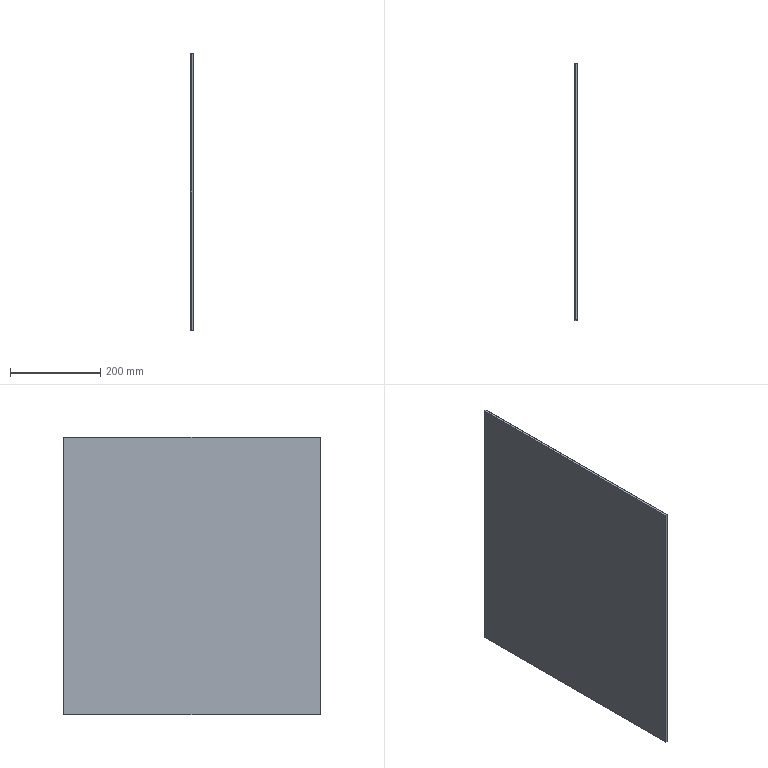Part | STEP file | 01-09 Base frame seal plate 2 | 1 solid | 11 faces | box 5 x 570 x 615 mm | volume 180603 mm3 | plane 11
STEP:
#1=CARTESIAN_POINT('',(0.,0.,0.));
#2=DIRECTION('',(0.,0.,1.));
#3=DIRECTION('',(1.,0.,0.));
#4=AXIS2_PLACEMENT_3D('',#1,#2,#3);
#5=CARTESIAN_POINT('',(5.,0.,0.));
#6=VERTEX_POINT('',#5);
#7=CARTESIAN_POINT('',(0.,0.,0.));
#8=VERTEX_POINT('',#7);
#9=CARTESIAN_POINT('',(2.5,0.,0.));
#10=DIRECTION('',(-1.,0.,0.));
#11=VECTOR('',#10,1.);
#12=LINE('',#9,#11);
#13=CARTESIAN_POINT('',(5.,0.,0.));
#14=DIRECTION('',(0.,0.,-1.));
#15=DIRECTION('',(-1.,0.,0.));
#16=AXIS2_PLACEMENT_3D('',#13,#14,#15);
#17=PLANE('',#16);
#18=CARTESIAN_POINT('',(2.5,0.));
#19=DIRECTION('',(1.,0.));
#20=VECTOR('',#19,1.);
#21=LINE('',#18,#20);
#22=(GEOMETRIC_REPRESENTATION_CONTEXT(2)PARAMETRIC_REPRESENTATION_CONTEXT()REPRESENTATION_CONTEXT('',''));
#23=DEFINITIONAL_REPRESENTATION('',(#21),#22);
#24=PCURVE('',#17,#23);
#25=CARTESIAN_POINT('',(0.,0.,-615.));
#26=DIRECTION('',(0.,1.,0.));
#27=DIRECTION('',(0.,0.,1.));
#28=AXIS2_PLACEMENT_3D('',#25,#26,#27);
#29=PLANE('',#28);
#30=CARTESIAN_POINT('',(615.,2.5));
#31=DIRECTION('',(0.,-1.));
#32=VECTOR('',#31,1.);
#33=LINE('',#30,#32);
#34=(GEOMETRIC_REPRESENTATION_CONTEXT(2)PARAMETRIC_REPRESENTATION_CONTEXT()REPRESENTATION_CONTEXT('',''));
#35=DEFINITIONAL_REPRESENTATION('',(#33),#34);
#36=PCURVE('',#29,#35);
#37=SURFACE_CURVE('',#12,(#24,#36),.PCURVE_S1.);
#38=EDGE_CURVE('',#6,#8,#37,.T.);
#39=ORIENTED_EDGE('',*,*,#38,.F.);
#40=CARTESIAN_POINT('',(5.,570.,0.));
#41=VERTEX_POINT('',#40);
#42=CARTESIAN_POINT('',(5.,285.,0.));
#43=DIRECTION('',(0.,-1.,0.));
#44=VECTOR('',#43,1.);
#45=LINE('',#42,#44);
#46=CARTESIAN_POINT('',(0.,285.));
#47=DIRECTION('',(0.,-1.));
#48=VECTOR('',#47,1.);
#49=LINE('',#46,#48);
#50=(GEOMETRIC_REPRESENTATION_CONTEXT(2)PARAMETRIC_REPRESENTATION_CONTEXT()REPRESENTATION_CONTEXT('',''));
#51=DEFINITIONAL_REPRESENTATION('',(#49),#50);
#52=PCURVE('',#17,#51);
#53=CARTESIAN_POINT('',(5.,0.,-615.));
#54=DIRECTION('',(-1.,0.,0.));
#55=DIRECTION('',(0.,0.,1.));
#56=AXIS2_PLACEMENT_3D('',#53,#54,#55);
#57=PLANE('',#56);
#58=CARTESIAN_POINT('',(615.,285.));
#59=DIRECTION('',(0.,-1.));
#60=VECTOR('',#59,1.);
#61=LINE('',#58,#60);
#62=(GEOMETRIC_REPRESENTATION_CONTEXT(2)PARAMETRIC_REPRESENTATION_CONTEXT()REPRESENTATION_CONTEXT('',''));
#63=DEFINITIONAL_REPRESENTATION('',(#61),#62);
#64=PCURVE('',#57,#63);
#65=SURFACE_CURVE('',#45,(#52,#64),.PCURVE_S1.);
#66=EDGE_CURVE('',#41,#6,#65,.T.);
#67=ORIENTED_EDGE('',*,*,#66,.F.);
#68=CARTESIAN_POINT('',(0.,570.,0.));
#69=VERTEX_POINT('',#68);
#70=CARTESIAN_POINT('',(2.5,570.,0.));
#71=DIRECTION('',(1.,0.,0.));
#72=VECTOR('',#71,1.);
#73=LINE('',#70,#72);
#74=CARTESIAN_POINT('',(2.5,570.));
#75=DIRECTION('',(-1.,0.));
#76=VECTOR('',#75,1.);
#77=LINE('',#74,#76);
#78=(GEOMETRIC_REPRESENTATION_CONTEXT(2)PARAMETRIC_REPRESENTATION_CONTEXT()REPRESENTATION_CONTEXT('',''));
#79=DEFINITIONAL_REPRESENTATION('',(#77),#78);
#80=PCURVE('',#17,#79);
#81=CARTESIAN_POINT('',(0.,570.,0.));
#82=DIRECTION('',(0.,-1.,0.));
#83=DIRECTION('',(0.,0.,-1.));
#84=AXIS2_PLACEMENT_3D('',#81,#82,#83);
#85=PLANE('',#84);
#86=CARTESIAN_POINT('',(0.,2.5));
#87=DIRECTION('',(0.,1.));
#88=VECTOR('',#87,1.);
#89=LINE('',#86,#88);
#90=(GEOMETRIC_REPRESENTATION_CONTEXT(2)PARAMETRIC_REPRESENTATION_CONTEXT()REPRESENTATION_CONTEXT('',''));
#91=DEFINITIONAL_REPRESENTATION('',(#89),#90);
#92=PCURVE('',#85,#91);
#93=SURFACE_CURVE('',#73,(#80,#92),.PCURVE_S1.);
#94=EDGE_CURVE('',#69,#41,#93,.T.);
#95=ORIENTED_EDGE('',*,*,#94,.F.);
#96=CARTESIAN_POINT('',(0.,285.,0.));
#97=DIRECTION('',(0.,1.,0.));
#98=VECTOR('',#97,1.);
#99=LINE('',#96,#98);
#100=CARTESIAN_POINT('',(5.,285.));
#101=DIRECTION('',(0.,1.));
#102=VECTOR('',#101,1.);
#103=LINE('',#100,#102);
#104=(GEOMETRIC_REPRESENTATION_CONTEXT(2)PARAMETRIC_REPRESENTATION_CONTEXT()REPRESENTATION_CONTEXT('',''));
#105=DEFINITIONAL_REPRESENTATION('',(#103),#104);
#106=PCURVE('',#17,#105);
#107=CARTESIAN_POINT('',(0.,0.,-615.));
#108=DIRECTION('',(-1.,0.,0.));
#109=DIRECTION('',(0.,0.,1.));
#110=AXIS2_PLACEMENT_3D('',#107,#108,#109);
#111=PLANE('',#110);
#112=CARTESIAN_POINT('',(615.,285.));
#113=DIRECTION('',(0.,1.));
#114=VECTOR('',#113,1.);
#115=LINE('',#112,#114);
#116=(GEOMETRIC_REPRESENTATION_CONTEXT(2)PARAMETRIC_REPRESENTATION_CONTEXT()REPRESENTATION_CONTEXT('',''));
#117=DEFINITIONAL_REPRESENTATION('',(#115),#116);
#118=PCURVE('',#111,#117);
#119=SURFACE_CURVE('',#99,(#106,#118),.PCURVE_S1.);
#120=EDGE_CURVE('',#8,#69,#119,.T.);
#121=ORIENTED_EDGE('',*,*,#120,.F.);
#122=EDGE_LOOP('',(#39,#67,#95,#121));
#123=FACE_BOUND('',#122,.T.);
#124=ADVANCED_FACE('',(#123),#17,.F.);
#125=CARTESIAN_POINT('',(0.,570.,-615.));
#126=VERTEX_POINT('',#125);
#127=CARTESIAN_POINT('',(0.,0.,-615.));
#128=VERTEX_POINT('',#127);
#129=CARTESIAN_POINT('',(0.,285.,-615.));
#130=DIRECTION('',(0.,-1.,0.));
#131=VECTOR('',#130,1.);
#132=LINE('',#129,#131);
#133=CARTESIAN_POINT('',(0.,285.));
#134=DIRECTION('',(0.,-1.));
#135=VECTOR('',#134,1.);
#136=LINE('',#133,#135);
#137=(GEOMETRIC_REPRESENTATION_CONTEXT(2)PARAMETRIC_REPRESENTATION_CONTEXT()REPRESENTATION_CONTEXT('',''));
#138=DEFINITIONAL_REPRESENTATION('',(#136),#137);
#139=PCURVE('',#111,#138);
#140=CARTESIAN_POINT('',(0.,0.,-615.));
#141=DIRECTION('',(0.,0.,1.));
#142=DIRECTION('',(1.,0.,0.));
#143=AXIS2_PLACEMENT_3D('',#140,#141,#142);
#144=PLANE('',#143);
#145=CARTESIAN_POINT('',(0.,285.));
#146=DIRECTION('',(0.,-1.));
#147=VECTOR('',#146,1.);
#148=LINE('',#145,#147);
#149=(GEOMETRIC_REPRESENTATION_CONTEXT(2)PARAMETRIC_REPRESENTATION_CONTEXT()REPRESENTATION_CONTEXT('',''));
#150=DEFINITIONAL_REPRESENTATION('',(#148),#149);
#151=PCURVE('',#144,#150);
#152=SURFACE_CURVE('',#132,(#139,#151),.PCURVE_S1.);
#153=EDGE_CURVE('',#126,#128,#152,.T.);
#154=ORIENTED_EDGE('',*,*,#153,.T.);
#155=CARTESIAN_POINT('',(0.,0.,-307.5));
#156=DIRECTION('',(0.,0.,1.));
#157=VECTOR('',#156,1.);
#158=LINE('',#155,#157);
#159=CARTESIAN_POINT('',(307.5,0.));
#160=DIRECTION('',(1.,0.));
#161=VECTOR('',#160,1.);
#162=LINE('',#159,#161);
#163=(GEOMETRIC_REPRESENTATION_CONTEXT(2)PARAMETRIC_REPRESENTATION_CONTEXT()REPRESENTATION_CONTEXT('',''));
#164=DEFINITIONAL_REPRESENTATION('',(#162),#163);
#165=PCURVE('',#111,#164);
#166=CARTESIAN_POINT('',(307.5,0.));
#167=DIRECTION('',(1.,0.));
#168=VECTOR('',#167,1.);
#169=LINE('',#166,#168);
#170=(GEOMETRIC_REPRESENTATION_CONTEXT(2)PARAMETRIC_REPRESENTATION_CONTEXT()REPRESENTATION_CONTEXT('',''));
#171=DEFINITIONAL_REPRESENTATION('',(#169),#170);
#172=PCURVE('',#29,#171);
#173=SURFACE_CURVE('',#158,(#165,#172),.PCURVE_S1.);
#174=EDGE_CURVE('',#128,#8,#173,.T.);
#175=ORIENTED_EDGE('',*,*,#174,.T.);
#176=ORIENTED_EDGE('',*,*,#120,.T.);
#177=CARTESIAN_POINT('',(0.,570.,-307.5));
#178=DIRECTION('',(0.,0.,-1.));
#179=VECTOR('',#178,1.);
#180=LINE('',#177,#179);
#181=CARTESIAN_POINT('',(307.5,570.));
#182=DIRECTION('',(-1.,0.));
#183=VECTOR('',#182,1.);
#184=LINE('',#181,#183);
#185=(GEOMETRIC_REPRESENTATION_CONTEXT(2)PARAMETRIC_REPRESENTATION_CONTEXT()REPRESENTATION_CONTEXT('',''));
#186=DEFINITIONAL_REPRESENTATION('',(#184),#185);
#187=PCURVE('',#111,#186);
#188=CARTESIAN_POINT('',(307.5,0.));
#189=DIRECTION('',(1.,0.));
#190=VECTOR('',#189,1.);
#191=LINE('',#188,#190);
#192=(GEOMETRIC_REPRESENTATION_CONTEXT(2)PARAMETRIC_REPRESENTATION_CONTEXT()REPRESENTATION_CONTEXT('',''));
#193=DEFINITIONAL_REPRESENTATION('',(#191),#192);
#194=PCURVE('',#85,#193);
#195=SURFACE_CURVE('',#180,(#187,#194),.PCURVE_S1.);
#196=EDGE_CURVE('',#69,#126,#195,.T.);
#197=ORIENTED_EDGE('',*,*,#196,.T.);
#198=EDGE_LOOP('',(#154,#175,#176,#197));
#199=FACE_BOUND('',#198,.T.);
#200=ADVANCED_FACE('',(#199),#111,.T.);
#201=CARTESIAN_POINT('',(5.,0.,-615.));
#202=VERTEX_POINT('',#201);
#203=CARTESIAN_POINT('',(2.5,0.,-615.));
#204=DIRECTION('',(-1.,0.,0.));
#205=VECTOR('',#204,1.);
#206=LINE('',#203,#205);
#207=CARTESIAN_POINT('',(0.,2.5));
#208=DIRECTION('',(0.,-1.));
#209=VECTOR('',#208,1.);
#210=LINE('',#207,#209);
#211=(GEOMETRIC_REPRESENTATION_CONTEXT(2)PARAMETRIC_REPRESENTATION_CONTEXT()REPRESENTATION_CONTEXT('',''));
#212=DEFINITIONAL_REPRESENTATION('',(#210),#211);
#213=PCURVE('',#29,#212);
#214=CARTESIAN_POINT('',(2.5,0.));
#215=DIRECTION('',(-1.,0.));
#216=VECTOR('',#215,1.);
#217=LINE('',#214,#216);
#218=(GEOMETRIC_REPRESENTATION_CONTEXT(2)PARAMETRIC_REPRESENTATION_CONTEXT()REPRESENTATION_CONTEXT('',''));
#219=DEFINITIONAL_REPRESENTATION('',(#217),#218);
#220=PCURVE('',#144,#219);
#221=SURFACE_CURVE('',#206,(#213,#220),.PCURVE_S1.);
#222=EDGE_CURVE('',#202,#128,#221,.T.);
#223=ORIENTED_EDGE('',*,*,#222,.F.);
#224=CARTESIAN_POINT('',(5.,0.,-307.5));
#225=DIRECTION('',(0.,0.,-1.));
#226=VECTOR('',#225,1.);
#227=LINE('',#224,#226);
#228=CARTESIAN_POINT('',(307.5,5.));
#229=DIRECTION('',(-1.,0.));
#230=VECTOR('',#229,1.);
#231=LINE('',#228,#230);
#232=(GEOMETRIC_REPRESENTATION_CONTEXT(2)PARAMETRIC_REPRESENTATION_CONTEXT()REPRESENTATION_CONTEXT('',''));
#233=DEFINITIONAL_REPRESENTATION('',(#231),#232);
#234=PCURVE('',#29,#233);
#235=CARTESIAN_POINT('',(307.5,0.));
#236=DIRECTION('',(-1.,0.));
#237=VECTOR('',#236,1.);
#238=LINE('',#235,#237);
#239=(GEOMETRIC_REPRESENTATION_CONTEXT(2)PARAMETRIC_REPRESENTATION_CONTEXT()REPRESENTATION_CONTEXT('',''));
#240=DEFINITIONAL_REPRESENTATION('',(#238),#239);
#241=PCURVE('',#57,#240);
#242=SURFACE_CURVE('',#227,(#234,#241),.PCURVE_S1.);
#243=EDGE_CURVE('',#6,#202,#242,.T.);
#244=ORIENTED_EDGE('',*,*,#243,.F.);
#245=ORIENTED_EDGE('',*,*,#38,.T.);
#246=ORIENTED_EDGE('',*,*,#174,.F.);
#247=EDGE_LOOP('',(#223,#244,#245,#246));
#248=FACE_BOUND('',#247,.T.);
#249=ADVANCED_FACE('',(#248),#29,.F.);
#250=CARTESIAN_POINT('',(5.,0.5,-614.5));
#251=VERTEX_POINT('',#250);
#252=CARTESIAN_POINT('',(5.,569.5,-614.5));
#253=VERTEX_POINT('',#252);
#254=CARTESIAN_POINT('',(5.,285.,-614.5));
#255=DIRECTION('',(0.,1.,0.));
#256=VECTOR('',#255,1.);
#257=LINE('',#254,#256);
#258=CARTESIAN_POINT('',(0.5,285.));
#259=DIRECTION('',(0.,1.));
#260=VECTOR('',#259,1.);
#261=LINE('',#258,#260);
#262=(GEOMETRIC_REPRESENTATION_CONTEXT(2)PARAMETRIC_REPRESENTATION_CONTEXT()REPRESENTATION_CONTEXT('',''));
#263=DEFINITIONAL_REPRESENTATION('',(#261),#262);
#264=PCURVE('',#57,#263);
#265=CARTESIAN_POINT('',(0.5,0.5,-614.5));
#266=DIRECTION('',(0.,0.,-1.));
#267=DIRECTION('',(0.,1.,0.));
#268=AXIS2_PLACEMENT_3D('',#265,#266,#267);
#269=PLANE('',#268);
#270=CARTESIAN_POINT('',(284.5,4.5));
#271=DIRECTION('',(1.,0.));
#272=VECTOR('',#271,1.);
#273=LINE('',#270,#272);
#274=(GEOMETRIC_REPRESENTATION_CONTEXT(2)PARAMETRIC_REPRESENTATION_CONTEXT()REPRESENTATION_CONTEXT('',''));
#275=DEFINITIONAL_REPRESENTATION('',(#273),#274);
#276=PCURVE('',#269,#275);
#277=SURFACE_CURVE('',#257,(#264,#276),.PCURVE_S1.);
#278=EDGE_CURVE('',#251,#253,#277,.T.);
#279=ORIENTED_EDGE('',*,*,#278,.F.);
#280=CARTESIAN_POINT('',(5.,0.5,-0.5));
#281=VERTEX_POINT('',#280);
#282=CARTESIAN_POINT('',(5.,0.5,-307.5));
#283=DIRECTION('',(0.,0.,-1.));
#284=VECTOR('',#283,1.);
#285=LINE('',#282,#284);
#286=CARTESIAN_POINT('',(307.5,0.5));
#287=DIRECTION('',(-1.,0.));
#288=VECTOR('',#287,1.);
#289=LINE('',#286,#288);
#290=(GEOMETRIC_REPRESENTATION_CONTEXT(2)PARAMETRIC_REPRESENTATION_CONTEXT()REPRESENTATION_CONTEXT('',''));
#291=DEFINITIONAL_REPRESENTATION('',(#289),#290);
#292=PCURVE('',#57,#291);
#293=CARTESIAN_POINT('',(0.5,0.5,-0.5));
#294=DIRECTION('',(0.,-1.,0.));
#295=DIRECTION('',(0.,0.,-1.));
#296=AXIS2_PLACEMENT_3D('',#293,#294,#295);
#297=PLANE('',#296);
#298=CARTESIAN_POINT('',(307.,4.5));
#299=DIRECTION('',(1.,0.));
#300=VECTOR('',#299,1.);
#301=LINE('',#298,#300);
#302=(GEOMETRIC_REPRESENTATION_CONTEXT(2)PARAMETRIC_REPRESENTATION_CONTEXT()REPRESENTATION_CONTEXT('',''));
#303=DEFINITIONAL_REPRESENTATION('',(#301),#302);
#304=PCURVE('',#297,#303);
#305=SURFACE_CURVE('',#285,(#292,#304),.PCURVE_S1.);
#306=EDGE_CURVE('',#281,#251,#305,.T.);
#307=ORIENTED_EDGE('',*,*,#306,.F.);
#308=CARTESIAN_POINT('',(5.,569.5,-0.5));
#309=VERTEX_POINT('',#308);
#310=CARTESIAN_POINT('',(5.,285.,-0.5));
#311=DIRECTION('',(0.,-1.,0.));
#312=VECTOR('',#311,1.);
#313=LINE('',#310,#312);
#314=CARTESIAN_POINT('',(614.5,285.));
#315=DIRECTION('',(0.,-1.));
#316=VECTOR('',#315,1.);
#317=LINE('',#314,#316);
#318=(GEOMETRIC_REPRESENTATION_CONTEXT(2)PARAMETRIC_REPRESENTATION_CONTEXT()REPRESENTATION_CONTEXT('',''));
#319=DEFINITIONAL_REPRESENTATION('',(#317),#318);
#320=PCURVE('',#57,#319);
#321=CARTESIAN_POINT('',(0.5,569.5,-0.5));
#322=DIRECTION('',(0.,0.,1.));
#323=DIRECTION('',(0.,-1.,0.));
#324=AXIS2_PLACEMENT_3D('',#321,#322,#323);
#325=PLANE('',#324);
#326=CARTESIAN_POINT('',(284.5,4.5));
#327=DIRECTION('',(1.,0.));
#328=VECTOR('',#327,1.);
#329=LINE('',#326,#328);
#330=(GEOMETRIC_REPRESENTATION_CONTEXT(2)PARAMETRIC_REPRESENTATION_CONTEXT()REPRESENTATION_CONTEXT('',''));
#331=DEFINITIONAL_REPRESENTATION('',(#329),#330);
#332=PCURVE('',#325,#331);
#333=SURFACE_CURVE('',#313,(#320,#332),.PCURVE_S1.);
#334=EDGE_CURVE('',#309,#281,#333,.T.);
#335=ORIENTED_EDGE('',*,*,#334,.F.);
#336=CARTESIAN_POINT('',(5.,569.5,-307.5));
#337=DIRECTION('',(0.,0.,1.));
#338=VECTOR('',#337,1.);
#339=LINE('',#336,#338);
#340=CARTESIAN_POINT('',(307.5,569.5));
#341=DIRECTION('',(1.,0.));
#342=VECTOR('',#341,1.);
#343=LINE('',#340,#342);
#344=(GEOMETRIC_REPRESENTATION_CONTEXT(2)PARAMETRIC_REPRESENTATION_CONTEXT()REPRESENTATION_CONTEXT('',''));
#345=DEFINITIONAL_REPRESENTATION('',(#343),#344);
#346=PCURVE('',#57,#345);
#347=CARTESIAN_POINT('',(0.5,569.5,-614.5));
#348=DIRECTION('',(0.,1.,0.));
#349=DIRECTION('',(0.,0.,1.));
#350=AXIS2_PLACEMENT_3D('',#347,#348,#349);
#351=PLANE('',#350);
#352=CARTESIAN_POINT('',(307.,4.5));
#353=DIRECTION('',(1.,0.));
#354=VECTOR('',#353,1.);
#355=LINE('',#352,#354);
#356=(GEOMETRIC_REPRESENTATION_CONTEXT(2)PARAMETRIC_REPRESENTATION_CONTEXT()REPRESENTATION_CONTEXT('',''));
#357=DEFINITIONAL_REPRESENTATION('',(#355),#356);
#358=PCURVE('',#351,#357);
#359=SURFACE_CURVE('',#339,(#346,#358),.PCURVE_S1.);
#360=EDGE_CURVE('',#253,#309,#359,.T.);
#361=ORIENTED_EDGE('',*,*,#360,.F.);
#362=EDGE_LOOP('',(#279,#307,#335,#361));
#363=FACE_BOUND('',#362,.T.);
#364=CARTESIAN_POINT('',(5.,570.,-615.));
#365=VERTEX_POINT('',#364);
#366=CARTESIAN_POINT('',(5.,570.,-307.5));
#367=DIRECTION('',(0.,0.,-1.));
#368=VECTOR('',#367,1.);
#369=LINE('',#366,#368);
#370=CARTESIAN_POINT('',(307.5,570.));
#371=DIRECTION('',(-1.,0.));
#372=VECTOR('',#371,1.);
#373=LINE('',#370,#372);
#374=(GEOMETRIC_REPRESENTATION_CONTEXT(2)PARAMETRIC_REPRESENTATION_CONTEXT()REPRESENTATION_CONTEXT('',''));
#375=DEFINITIONAL_REPRESENTATION('',(#373),#374);
#376=PCURVE('',#57,#375);
#377=CARTESIAN_POINT('',(307.5,5.));
#378=DIRECTION('',(1.,0.));
#379=VECTOR('',#378,1.);
#380=LINE('',#377,#379);
#381=(GEOMETRIC_REPRESENTATION_CONTEXT(2)PARAMETRIC_REPRESENTATION_CONTEXT()REPRESENTATION_CONTEXT('',''));
#382=DEFINITIONAL_REPRESENTATION('',(#380),#381);
#383=PCURVE('',#85,#382);
#384=SURFACE_CURVE('',#369,(#376,#383),.PCURVE_S1.);
#385=EDGE_CURVE('',#41,#365,#384,.T.);
#386=ORIENTED_EDGE('',*,*,#385,.F.);
#387=ORIENTED_EDGE('',*,*,#66,.T.);
#388=ORIENTED_EDGE('',*,*,#243,.T.);
#389=CARTESIAN_POINT('',(5.,285.,-615.));
#390=DIRECTION('',(0.,-1.,0.));
#391=VECTOR('',#390,1.);
#392=LINE('',#389,#391);
#393=CARTESIAN_POINT('',(0.,285.));
#394=DIRECTION('',(0.,-1.));
#395=VECTOR('',#394,1.);
#396=LINE('',#393,#395);
#397=(GEOMETRIC_REPRESENTATION_CONTEXT(2)PARAMETRIC_REPRESENTATION_CONTEXT()REPRESENTATION_CONTEXT('',''));
#398=DEFINITIONAL_REPRESENTATION('',(#396),#397);
#399=PCURVE('',#57,#398);
#400=CARTESIAN_POINT('',(5.,285.));
#401=DIRECTION('',(0.,-1.));
#402=VECTOR('',#401,1.);
#403=LINE('',#400,#402);
#404=(GEOMETRIC_REPRESENTATION_CONTEXT(2)PARAMETRIC_REPRESENTATION_CONTEXT()REPRESENTATION_CONTEXT('',''));
#405=DEFINITIONAL_REPRESENTATION('',(#403),#404);
#406=PCURVE('',#144,#405);
#407=SURFACE_CURVE('',#392,(#399,#406),.PCURVE_S1.);
#408=EDGE_CURVE('',#365,#202,#407,.T.);
#409=ORIENTED_EDGE('',*,*,#408,.F.);
#410=EDGE_LOOP('',(#386,#387,#388,#409));
#411=FACE_BOUND('',#410,.T.);
#412=ADVANCED_FACE('',(#363,#411),#57,.F.);
#413=ORIENTED_EDGE('',*,*,#94,.T.);
#414=ORIENTED_EDGE('',*,*,#385,.T.);
#415=CARTESIAN_POINT('',(2.5,570.,-615.));
#416=DIRECTION('',(1.,0.,0.));
#417=VECTOR('',#416,1.);
#418=LINE('',#415,#417);
#419=CARTESIAN_POINT('',(615.,2.5));
#420=DIRECTION('',(0.,1.));
#421=VECTOR('',#420,1.);
#422=LINE('',#419,#421);
#423=(GEOMETRIC_REPRESENTATION_CONTEXT(2)PARAMETRIC_REPRESENTATION_CONTEXT()REPRESENTATION_CONTEXT('',''));
#424=DEFINITIONAL_REPRESENTATION('',(#422),#423);
#425=PCURVE('',#85,#424);
#426=CARTESIAN_POINT('',(2.5,570.));
#427=DIRECTION('',(1.,0.));
#428=VECTOR('',#427,1.);
#429=LINE('',#426,#428);
#430=(GEOMETRIC_REPRESENTATION_CONTEXT(2)PARAMETRIC_REPRESENTATION_CONTEXT()REPRESENTATION_CONTEXT('',''));
#431=DEFINITIONAL_REPRESENTATION('',(#429),#430);
#432=PCURVE('',#144,#431);
#433=SURFACE_CURVE('',#418,(#425,#432),.PCURVE_S1.);
#434=EDGE_CURVE('',#126,#365,#433,.T.);
#435=ORIENTED_EDGE('',*,*,#434,.F.);
#436=ORIENTED_EDGE('',*,*,#196,.F.);
#437=EDGE_LOOP('',(#413,#414,#435,#436));
#438=FACE_BOUND('',#437,.T.);
#439=ADVANCED_FACE('',(#438),#85,.F.);
#440=ORIENTED_EDGE('',*,*,#434,.T.);
#441=ORIENTED_EDGE('',*,*,#408,.T.);
#442=ORIENTED_EDGE('',*,*,#222,.T.);
#443=ORIENTED_EDGE('',*,*,#153,.F.);
#444=EDGE_LOOP('',(#440,#441,#442,#443));
#445=FACE_BOUND('',#444,.T.);
#446=ADVANCED_FACE('',(#445),#144,.F.);
#447=CARTESIAN_POINT('',(0.5,569.5,-614.5));
#448=VERTEX_POINT('',#447);
#449=CARTESIAN_POINT('',(0.5,569.5,-0.5));
#450=VERTEX_POINT('',#449);
#451=CARTESIAN_POINT('',(0.5,569.5,-307.5));
#452=DIRECTION('',(0.,0.,1.));
#453=VECTOR('',#452,1.);
#454=LINE('',#451,#453);
#455=CARTESIAN_POINT('',(307.,0.));
#456=DIRECTION('',(1.,0.));
#457=VECTOR('',#456,1.);
#458=LINE('',#455,#457);
#459=(GEOMETRIC_REPRESENTATION_CONTEXT(2)PARAMETRIC_REPRESENTATION_CONTEXT()REPRESENTATION_CONTEXT('',''));
#460=DEFINITIONAL_REPRESENTATION('',(#458),#459);
#461=PCURVE('',#351,#460);
#462=CARTESIAN_POINT('',(0.5,0.5,-614.5));
#463=DIRECTION('',(-1.,0.,0.));
#464=DIRECTION('',(0.,0.,1.));
#465=AXIS2_PLACEMENT_3D('',#462,#463,#464);
#466=PLANE('',#465);
#467=CARTESIAN_POINT('',(307.,569.));
#468=DIRECTION('',(1.,0.));
#469=VECTOR('',#468,1.);
#470=LINE('',#467,#469);
#471=(GEOMETRIC_REPRESENTATION_CONTEXT(2)PARAMETRIC_REPRESENTATION_CONTEXT()REPRESENTATION_CONTEXT('',''));
#472=DEFINITIONAL_REPRESENTATION('',(#470),#471);
#473=PCURVE('',#466,#472);
#474=SURFACE_CURVE('',#454,(#461,#473),.PCURVE_S1.);
#475=EDGE_CURVE('',#448,#450,#474,.T.);
#476=ORIENTED_EDGE('',*,*,#475,.F.);
#477=CARTESIAN_POINT('',(2.75,569.5,-614.5));
#478=DIRECTION('',(-1.,0.,0.));
#479=VECTOR('',#478,1.);
#480=LINE('',#477,#479);
#481=CARTESIAN_POINT('',(0.,2.25));
#482=DIRECTION('',(0.,-1.));
#483=VECTOR('',#482,1.);
#484=LINE('',#481,#483);
#485=(GEOMETRIC_REPRESENTATION_CONTEXT(2)PARAMETRIC_REPRESENTATION_CONTEXT()REPRESENTATION_CONTEXT('',''));
#486=DEFINITIONAL_REPRESENTATION('',(#484),#485);
#487=PCURVE('',#351,#486);
#488=CARTESIAN_POINT('',(569.,2.25));
#489=DIRECTION('',(0.,-1.));
#490=VECTOR('',#489,1.);
#491=LINE('',#488,#490);
#492=(GEOMETRIC_REPRESENTATION_CONTEXT(2)PARAMETRIC_REPRESENTATION_CONTEXT()REPRESENTATION_CONTEXT('',''));
#493=DEFINITIONAL_REPRESENTATION('',(#491),#492);
#494=PCURVE('',#269,#493);
#495=SURFACE_CURVE('',#480,(#487,#494),.PCURVE_S1.);
#496=EDGE_CURVE('',#253,#448,#495,.T.);
#497=ORIENTED_EDGE('',*,*,#496,.F.);
#498=ORIENTED_EDGE('',*,*,#360,.T.);
#499=CARTESIAN_POINT('',(2.75,569.5,-0.5));
#500=DIRECTION('',(1.,0.,0.));
#501=VECTOR('',#500,1.);
#502=LINE('',#499,#501);
#503=CARTESIAN_POINT('',(614.,2.25));
#504=DIRECTION('',(0.,1.));
#505=VECTOR('',#504,1.);
#506=LINE('',#503,#505);
#507=(GEOMETRIC_REPRESENTATION_CONTEXT(2)PARAMETRIC_REPRESENTATION_CONTEXT()REPRESENTATION_CONTEXT('',''));
#508=DEFINITIONAL_REPRESENTATION('',(#506),#507);
#509=PCURVE('',#351,#508);
#510=CARTESIAN_POINT('',(0.,2.25));
#511=DIRECTION('',(0.,1.));
#512=VECTOR('',#511,1.);
#513=LINE('',#510,#512);
#514=(GEOMETRIC_REPRESENTATION_CONTEXT(2)PARAMETRIC_REPRESENTATION_CONTEXT()REPRESENTATION_CONTEXT('',''));
#515=DEFINITIONAL_REPRESENTATION('',(#513),#514);
#516=PCURVE('',#325,#515);
#517=SURFACE_CURVE('',#502,(#509,#516),.PCURVE_S1.);
#518=EDGE_CURVE('',#450,#309,#517,.T.);
#519=ORIENTED_EDGE('',*,*,#518,.F.);
#520=EDGE_LOOP('',(#476,#497,#498,#519));
#521=FACE_BOUND('',#520,.T.);
#522=ADVANCED_FACE('',(#521),#351,.F.);
#523=CARTESIAN_POINT('',(0.5,0.5,-614.5));
#524=VERTEX_POINT('',#523);
#525=CARTESIAN_POINT('',(0.5,285.,-614.5));
#526=DIRECTION('',(0.,1.,0.));
#527=VECTOR('',#526,1.);
#528=LINE('',#525,#527);
#529=CARTESIAN_POINT('',(284.5,0.));
#530=DIRECTION('',(1.,0.));
#531=VECTOR('',#530,1.);
#532=LINE('',#529,#531);
#533=(GEOMETRIC_REPRESENTATION_CONTEXT(2)PARAMETRIC_REPRESENTATION_CONTEXT()REPRESENTATION_CONTEXT('',''));
#534=DEFINITIONAL_REPRESENTATION('',(#532),#533);
#535=PCURVE('',#269,#534);
#536=CARTESIAN_POINT('',(0.,284.5));
#537=DIRECTION('',(0.,1.));
#538=VECTOR('',#537,1.);
#539=LINE('',#536,#538);
#540=(GEOMETRIC_REPRESENTATION_CONTEXT(2)PARAMETRIC_REPRESENTATION_CONTEXT()REPRESENTATION_CONTEXT('',''));
#541=DEFINITIONAL_REPRESENTATION('',(#539),#540);
#542=PCURVE('',#466,#541);
#543=SURFACE_CURVE('',#528,(#535,#542),.PCURVE_S1.);
#544=EDGE_CURVE('',#524,#448,#543,.T.);
#545=ORIENTED_EDGE('',*,*,#544,.F.);
#546=CARTESIAN_POINT('',(2.75,0.5,-614.5));
#547=DIRECTION('',(-1.,0.,0.));
#548=VECTOR('',#547,1.);
#549=LINE('',#546,#548);
#550=CARTESIAN_POINT('',(0.,2.25));
#551=DIRECTION('',(0.,-1.));
#552=VECTOR('',#551,1.);
#553=LINE('',#550,#552);
#554=(GEOMETRIC_REPRESENTATION_CONTEXT(2)PARAMETRIC_REPRESENTATION_CONTEXT()REPRESENTATION_CONTEXT('',''));
#555=DEFINITIONAL_REPRESENTATION('',(#553),#554);
#556=PCURVE('',#269,#555);
#557=CARTESIAN_POINT('',(614.,2.25));
#558=DIRECTION('',(0.,-1.));
#559=VECTOR('',#558,1.);
#560=LINE('',#557,#559);
#561=(GEOMETRIC_REPRESENTATION_CONTEXT(2)PARAMETRIC_REPRESENTATION_CONTEXT()REPRESENTATION_CONTEXT('',''));
#562=DEFINITIONAL_REPRESENTATION('',(#560),#561);
#563=PCURVE('',#297,#562);
#564=SURFACE_CURVE('',#549,(#556,#563),.PCURVE_S1.);
#565=EDGE_CURVE('',#251,#524,#564,.T.);
#566=ORIENTED_EDGE('',*,*,#565,.F.);
#567=ORIENTED_EDGE('',*,*,#278,.T.);
#568=ORIENTED_EDGE('',*,*,#496,.T.);
#569=EDGE_LOOP('',(#545,#566,#567,#568));
#570=FACE_BOUND('',#569,.T.);
#571=ADVANCED_FACE('',(#570),#269,.F.);
#572=CARTESIAN_POINT('',(0.5,0.5,-0.5));
#573=VERTEX_POINT('',#572);
#574=CARTESIAN_POINT('',(0.5,0.5,-307.5));
#575=DIRECTION('',(0.,0.,-1.));
#576=VECTOR('',#575,1.);
#577=LINE('',#574,#576);
#578=CARTESIAN_POINT('',(307.,0.));
#579=DIRECTION('',(1.,0.));
#580=VECTOR('',#579,1.);
#581=LINE('',#578,#580);
#582=(GEOMETRIC_REPRESENTATION_CONTEXT(2)PARAMETRIC_REPRESENTATION_CONTEXT()REPRESENTATION_CONTEXT('',''));
#583=DEFINITIONAL_REPRESENTATION('',(#581),#582);
#584=PCURVE('',#297,#583);
#585=CARTESIAN_POINT('',(307.,0.));
#586=DIRECTION('',(-1.,0.));
#587=VECTOR('',#586,1.);
#588=LINE('',#585,#587);
#589=(GEOMETRIC_REPRESENTATION_CONTEXT(2)PARAMETRIC_REPRESENTATION_CONTEXT()REPRESENTATION_CONTEXT('',''));
#590=DEFINITIONAL_REPRESENTATION('',(#588),#589);
#591=PCURVE('',#466,#590);
#592=SURFACE_CURVE('',#577,(#584,#591),.PCURVE_S1.);
#593=EDGE_CURVE('',#573,#524,#592,.T.);
#594=ORIENTED_EDGE('',*,*,#593,.F.);
#595=CARTESIAN_POINT('',(2.75,0.5,-0.5));
#596=DIRECTION('',(-1.,0.,0.));
#597=VECTOR('',#596,1.);
#598=LINE('',#595,#597);
#599=CARTESIAN_POINT('',(0.,2.25));
#600=DIRECTION('',(0.,-1.));
#601=VECTOR('',#600,1.);
#602=LINE('',#599,#601);
#603=(GEOMETRIC_REPRESENTATION_CONTEXT(2)PARAMETRIC_REPRESENTATION_CONTEXT()REPRESENTATION_CONTEXT('',''));
#604=DEFINITIONAL_REPRESENTATION('',(#602),#603);
#605=PCURVE('',#297,#604);
#606=CARTESIAN_POINT('',(569.,2.25));
#607=DIRECTION('',(0.,-1.));
#608=VECTOR('',#607,1.);
#609=LINE('',#606,#608);
#610=(GEOMETRIC_REPRESENTATION_CONTEXT(2)PARAMETRIC_REPRESENTATION_CONTEXT()REPRESENTATION_CONTEXT('',''));
#611=DEFINITIONAL_REPRESENTATION('',(#609),#610);
#612=PCURVE('',#325,#611);
#613=SURFACE_CURVE('',#598,(#605,#612),.PCURVE_S1.);
#614=EDGE_CURVE('',#281,#573,#613,.T.);
#615=ORIENTED_EDGE('',*,*,#614,.F.);
#616=ORIENTED_EDGE('',*,*,#306,.T.);
#617=ORIENTED_EDGE('',*,*,#565,.T.);
#618=EDGE_LOOP('',(#594,#615,#616,#617));
#619=FACE_BOUND('',#618,.T.);
#620=ADVANCED_FACE('',(#619),#297,.F.);
#621=CARTESIAN_POINT('',(0.5,285.,-0.5));
#622=DIRECTION('',(0.,-1.,0.));
#623=VECTOR('',#622,1.);
#624=LINE('',#621,#623);
#625=CARTESIAN_POINT('',(284.5,0.));
#626=DIRECTION('',(1.,0.));
#627=VECTOR('',#626,1.);
#628=LINE('',#625,#627);
#629=(GEOMETRIC_REPRESENTATION_CONTEXT(2)PARAMETRIC_REPRESENTATION_CONTEXT()REPRESENTATION_CONTEXT('',''));
#630=DEFINITIONAL_REPRESENTATION('',(#628),#629);
#631=PCURVE('',#325,#630);
#632=CARTESIAN_POINT('',(614.,284.5));
#633=DIRECTION('',(0.,-1.));
#634=VECTOR('',#633,1.);
#635=LINE('',#632,#634);
#636=(GEOMETRIC_REPRESENTATION_CONTEXT(2)PARAMETRIC_REPRESENTATION_CONTEXT()REPRESENTATION_CONTEXT('',''));
#637=DEFINITIONAL_REPRESENTATION('',(#635),#636);
#638=PCURVE('',#466,#637);
#639=SURFACE_CURVE('',#624,(#631,#638),.PCURVE_S1.);
#640=EDGE_CURVE('',#450,#573,#639,.T.);
#641=ORIENTED_EDGE('',*,*,#640,.F.);
#642=ORIENTED_EDGE('',*,*,#518,.T.);
#643=ORIENTED_EDGE('',*,*,#334,.T.);
#644=ORIENTED_EDGE('',*,*,#614,.T.);
#645=EDGE_LOOP('',(#641,#642,#643,#644));
#646=FACE_BOUND('',#645,.T.);
#647=ADVANCED_FACE('',(#646),#325,.F.);
#648=ORIENTED_EDGE('',*,*,#475,.T.);
#649=ORIENTED_EDGE('',*,*,#640,.T.);
#650=ORIENTED_EDGE('',*,*,#593,.T.);
#651=ORIENTED_EDGE('',*,*,#544,.T.);
#652=EDGE_LOOP('',(#648,#649,#650,#651));
#653=FACE_BOUND('',#652,.T.);
#654=ADVANCED_FACE('',(#653),#466,.F.);
#655=CLOSED_SHELL('',(#124,#200,#249,#412,#439,#446,#522,#571,#620,#647,#654));
#656=MANIFOLD_SOLID_BREP('',#655);
#657=(LENGTH_UNIT()NAMED_UNIT(*)SI_UNIT(.MILLI.,.METRE.));
#658=UNCERTAINTY_MEASURE_WITH_UNIT(LENGTH_MEASURE(0.0000001),#657,'','');
#659=(NAMED_UNIT(*)PLANE_ANGLE_UNIT()SI_UNIT($,.RADIAN.));
#660=(NAMED_UNIT(*)SI_UNIT($,.STERADIAN.)SOLID_ANGLE_UNIT());
#661=(GEOMETRIC_REPRESENTATION_CONTEXT(3)GLOBAL_UNCERTAINTY_ASSIGNED_CONTEXT((#658))GLOBAL_UNIT_ASSIGNED_CONTEXT((#657,#659,#660))REPRESENTATION_CONTEXT('',''));
#662=ADVANCED_BREP_SHAPE_REPRESENTATION('',(#4,#656),#661);